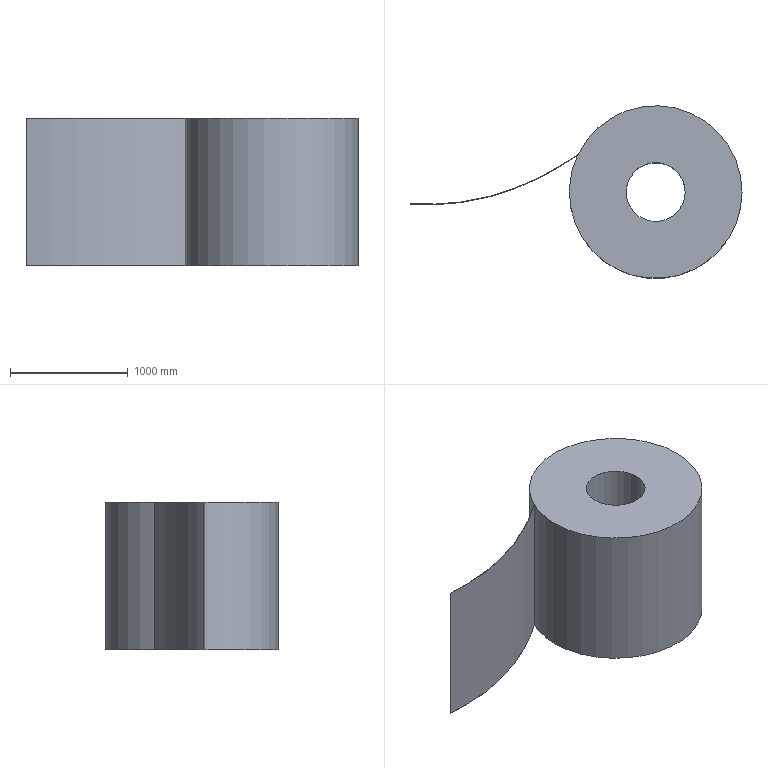Part | SolidWorks | features ExtruThin 1, ICE 1 | 1 solid | 10 faces | box 2820 x 1466 x 1250 mm | volume 1870768700 mm3 | cylinder 5 | plane 3 | spline 2 | commonest cylinder face diameters 1466 x3 500 x2
STEP:
#1=CARTESIAN_POINT('',(3099.7,210.,-625.));
#2=VERTEX_POINT('',#1);
#3=CARTESIAN_POINT('',(2599.7,210.,-625.));
#4=VERTEX_POINT('',#3);
#5=CARTESIAN_POINT('',(2849.7,210.,-625.));
#6=DIRECTION('',(0.,0.,-1.));
#7=DIRECTION('',(1.,0.,0.));
#8=AXIS2_PLACEMENT_3D('',#5,#6,#7);
#9=CIRCLE('',#8,250.);
#10=EDGE_CURVE('',#2,#4,#9,.T.);
#11=ORIENTED_EDGE('',*,*,#10,.T.);
#12=CARTESIAN_POINT('',(2599.7,210.,625.));
#13=VERTEX_POINT('',#12);
#14=CARTESIAN_POINT('',(2599.7,210.,-2698.525));
#15=DIRECTION('',(0.,0.,1.));
#16=VECTOR('',#15,1000.);
#17=LINE('',#14,#16);
#18=EDGE_CURVE('',#4,#13,#17,.T.);
#19=ORIENTED_EDGE('',*,*,#18,.T.);
#20=CARTESIAN_POINT('',(3099.7,210.,625.));
#21=VERTEX_POINT('',#20);
#22=CARTESIAN_POINT('',(2849.7,210.,625.));
#23=DIRECTION('',(0.,0.,1.));
#24=DIRECTION('',(1.,0.,0.));
#25=AXIS2_PLACEMENT_3D('',#22,#23,#24);
#26=CIRCLE('',#25,250.);
#27=EDGE_CURVE('',#13,#21,#26,.T.);
#28=ORIENTED_EDGE('',*,*,#27,.T.);
#29=CARTESIAN_POINT('',(3099.7,210.,-2698.525));
#30=DIRECTION('',(0.,0.,1.));
#31=VECTOR('',#30,1000.);
#32=LINE('',#29,#31);
#33=EDGE_CURVE('',#2,#21,#32,.T.);
#34=ORIENTED_EDGE('',*,*,#33,.F.);
#35=EDGE_LOOP('',(#11,#19,#28,#34));
#36=FACE_OUTER_BOUND('',#35,.T.);
#37=CARTESIAN_POINT('',(2849.7,210.,-2698.525));
#38=DIRECTION('',(0.,0.,1.));
#39=DIRECTION('',(1.,0.,0.));
#40=AXIS2_PLACEMENT_3D('',#37,#38,#39);
#41=CYLINDRICAL_SURFACE('',#40,250.);
#42=ADVANCED_FACE('',(#36),#41,.F.);
#43=CARTESIAN_POINT('',(2116.598,210.,-625.));
#44=VERTEX_POINT('',#43);
#45=CARTESIAN_POINT('',(2188.389,526.395,-625.));
#46=VERTEX_POINT('',#45);
#47=CARTESIAN_POINT('',(2849.7,210.,-625.));
#48=DIRECTION('',(0.,0.,-1.));
#49=DIRECTION('',(1.,0.,0.));
#50=AXIS2_PLACEMENT_3D('',#47,#48,#49);
#51=CIRCLE('',#50,733.102);
#52=EDGE_CURVE('',#44,#46,#51,.T.);
#53=ORIENTED_EDGE('',*,*,#52,.F.);
#54=CARTESIAN_POINT('',(2116.598,210.,625.));
#55=VERTEX_POINT('',#54);
#56=CARTESIAN_POINT('',(2116.598,210.,-2698.525));
#57=DIRECTION('',(0.,0.,1.));
#58=VECTOR('',#57,1000.);
#59=LINE('',#56,#58);
#60=EDGE_CURVE('',#44,#55,#59,.T.);
#61=ORIENTED_EDGE('',*,*,#60,.T.);
#62=CARTESIAN_POINT('',(2188.389,526.395,625.));
#63=VERTEX_POINT('',#62);
#64=CARTESIAN_POINT('',(2849.7,210.,625.));
#65=DIRECTION('',(0.,0.,1.));
#66=DIRECTION('',(1.,0.,0.));
#67=AXIS2_PLACEMENT_3D('',#64,#65,#66);
#68=CIRCLE('',#67,733.102);
#69=EDGE_CURVE('',#63,#55,#68,.T.);
#70=ORIENTED_EDGE('',*,*,#69,.F.);
#71=CARTESIAN_POINT('',(2188.389,526.395,625.));
#72=DIRECTION('',(0.,0.,1.));
#73=VECTOR('',#72,1000.);
#74=LINE('',#71,#73);
#75=EDGE_CURVE('',#46,#63,#74,.T.);
#76=ORIENTED_EDGE('',*,*,#75,.F.);
#77=EDGE_LOOP('',(#53,#61,#70,#76));
#78=FACE_OUTER_BOUND('',#77,.T.);
#79=CARTESIAN_POINT('',(2849.7,210.,-2698.525));
#80=DIRECTION('',(0.,0.,1.));
#81=DIRECTION('',(1.,0.,0.));
#82=AXIS2_PLACEMENT_3D('',#79,#80,#81);
#83=CYLINDRICAL_SURFACE('',#82,733.102);
#84=ADVANCED_FACE('',(#78),#83,.T.);
#85=ORIENTED_EDGE('',*,*,#60,.F.);
#86=CARTESIAN_POINT('',(3582.802,210.,-625.));
#87=VERTEX_POINT('',#86);
#88=CARTESIAN_POINT('',(2849.7,210.,-625.));
#89=DIRECTION('',(0.,0.,-1.));
#90=DIRECTION('',(1.,0.,0.));
#91=AXIS2_PLACEMENT_3D('',#88,#89,#90);
#92=CIRCLE('',#91,733.102);
#93=EDGE_CURVE('',#87,#44,#92,.T.);
#94=ORIENTED_EDGE('',*,*,#93,.F.);
#95=CARTESIAN_POINT('',(3582.802,210.,625.));
#96=VERTEX_POINT('',#95);
#97=CARTESIAN_POINT('',(3582.802,210.,-2698.525));
#98=DIRECTION('',(0.,0.,1.));
#99=VECTOR('',#98,1000.);
#100=LINE('',#97,#99);
#101=EDGE_CURVE('',#87,#96,#100,.T.);
#102=ORIENTED_EDGE('',*,*,#101,.T.);
#103=CARTESIAN_POINT('',(2849.7,210.,625.));
#104=DIRECTION('',(0.,0.,1.));
#105=DIRECTION('',(1.,0.,0.));
#106=AXIS2_PLACEMENT_3D('',#103,#104,#105);
#107=CIRCLE('',#106,733.102);
#108=EDGE_CURVE('',#55,#96,#107,.T.);
#109=ORIENTED_EDGE('',*,*,#108,.F.);
#110=EDGE_LOOP('',(#85,#94,#102,#109));
#111=FACE_OUTER_BOUND('',#110,.T.);
#112=CARTESIAN_POINT('',(2849.7,210.,-2698.525));
#113=DIRECTION('',(0.,0.,1.));
#114=DIRECTION('',(1.,0.,0.));
#115=AXIS2_PLACEMENT_3D('',#112,#113,#114);
#116=CYLINDRICAL_SURFACE('',#115,733.102);
#117=ADVANCED_FACE('',(#111),#116,.T.);
#118=CARTESIAN_POINT('',(762.74,109.82,-625.));
#119=VERTEX_POINT('',#118);
#120=CARTESIAN_POINT('',(762.74,109.82,-625.));
#121=CARTESIAN_POINT('',(1013.548,91.191,-625.));
#122=CARTESIAN_POINT('',(1258.171,116.87,-625.));
#123=CARTESIAN_POINT('',(1733.318,256.354,-625.));
#124=CARTESIAN_POINT('',(1963.927,369.542,-625.));
#125=CARTESIAN_POINT('',(2188.389,526.395,-625.));
#126=B_SPLINE_CURVE_WITH_KNOTS('',3,(#120,#121,#122,#123,#124,#125),.UNSPECIFIED.,.F.,.F.,(4,2,4),(0.,0.5,0.9965),.UNSPECIFIED.);
#127=EDGE_CURVE('',#119,#46,#126,.T.);
#128=ORIENTED_EDGE('',*,*,#127,.T.);
#129=ORIENTED_EDGE('',*,*,#75,.T.);
#130=CARTESIAN_POINT('',(762.74,109.82,625.));
#131=VERTEX_POINT('',#130);
#132=CARTESIAN_POINT('',(762.74,109.82,625.));
#133=CARTESIAN_POINT('',(1013.548,91.191,625.));
#134=CARTESIAN_POINT('',(1258.171,116.87,625.));
#135=CARTESIAN_POINT('',(1733.318,256.354,625.));
#136=CARTESIAN_POINT('',(1963.927,369.542,625.));
#137=CARTESIAN_POINT('',(2188.389,526.395,625.));
#138=B_SPLINE_CURVE_WITH_KNOTS('',3,(#132,#133,#134,#135,#136,#137),.UNSPECIFIED.,.F.,.F.,(4,2,4),(0.,0.5,0.9965),.UNSPECIFIED.);
#139=EDGE_CURVE('',#131,#63,#138,.T.);
#140=ORIENTED_EDGE('',*,*,#139,.F.);
#141=CARTESIAN_POINT('',(762.74,109.82,625.));
#142=DIRECTION('',(0.,0.,-1.));
#143=VECTOR('',#142,1000.);
#144=LINE('',#141,#143);
#145=EDGE_CURVE('',#131,#119,#144,.T.);
#146=ORIENTED_EDGE('',*,*,#145,.T.);
#147=EDGE_LOOP('',(#128,#129,#140,#146));
#148=FACE_OUTER_BOUND('',#147,.T.);
#149=CARTESIAN_POINT('',(762.74,109.82,625.));
#150=CARTESIAN_POINT('',(762.74,109.82,-625.));
#151=CARTESIAN_POINT('',(1013.548,91.191,625.));
#152=CARTESIAN_POINT('',(1013.548,91.191,-625.));
#153=CARTESIAN_POINT('',(1258.171,116.87,625.));
#154=CARTESIAN_POINT('',(1258.171,116.87,-625.));
#155=CARTESIAN_POINT('',(1733.318,256.354,625.));
#156=CARTESIAN_POINT('',(1733.318,256.354,-625.));
#157=CARTESIAN_POINT('',(1963.927,369.542,625.));
#158=CARTESIAN_POINT('',(1963.927,369.542,-625.));
#159=CARTESIAN_POINT('',(2188.389,526.395,625.));
#160=CARTESIAN_POINT('',(2188.389,526.395,-625.));
#161=B_SPLINE_SURFACE_WITH_KNOTS('',3,1,((#149,#150),(#151,#152),(#153,#154),(#155,#156),(#157,#158),(#159,#160)),.UNSPECIFIED.,.F.,.F.,.F.,(4,2,4),(2,2),(0.,0.5,0.9965),(0.,1.),.UNSPECIFIED.);
#162=ADVANCED_FACE('',(#148),#161,.F.);
#163=CARTESIAN_POINT('',(2191.067,531.933,-625.));
#164=VERTEX_POINT('',#163);
#165=CARTESIAN_POINT('',(2191.067,531.933,625.));
#166=VERTEX_POINT('',#165);
#167=CARTESIAN_POINT('',(2191.067,531.933,625.));
#168=DIRECTION('',(0.,0.,1.));
#169=VECTOR('',#168,1000.);
#170=LINE('',#167,#169);
#171=EDGE_CURVE('',#164,#166,#170,.T.);
#172=ORIENTED_EDGE('',*,*,#171,.F.);
#173=CARTESIAN_POINT('',(762.962,112.812,-625.));
#174=VERTEX_POINT('',#173);
#175=CARTESIAN_POINT('',(762.962,112.812,-625.));
#176=CARTESIAN_POINT('',(1013.423,94.209,-625.));
#177=CARTESIAN_POINT('',(1257.667,119.849,-625.));
#178=CARTESIAN_POINT('',(1733.679,259.586,-625.));
#179=CARTESIAN_POINT('',(1965.455,373.645,-625.));
#180=CARTESIAN_POINT('',(2191.067,531.933,-625.));
#181=B_SPLINE_CURVE_WITH_KNOTS('',3,(#175,#176,#177,#178,#179,#180),.UNSPECIFIED.,.F.,.F.,(4,2,4),(0.,0.5,0.9998),.UNSPECIFIED.);
#182=EDGE_CURVE('',#174,#164,#181,.T.);
#183=ORIENTED_EDGE('',*,*,#182,.F.);
#184=CARTESIAN_POINT('',(762.962,112.812,625.));
#185=VERTEX_POINT('',#184);
#186=CARTESIAN_POINT('',(762.962,112.812,625.));
#187=DIRECTION('',(0.,0.,-1.));
#188=VECTOR('',#187,1000.);
#189=LINE('',#186,#188);
#190=EDGE_CURVE('',#185,#174,#189,.T.);
#191=ORIENTED_EDGE('',*,*,#190,.F.);
#192=CARTESIAN_POINT('',(762.962,112.812,625.));
#193=CARTESIAN_POINT('',(1013.423,94.209,625.));
#194=CARTESIAN_POINT('',(1257.667,119.849,625.));
#195=CARTESIAN_POINT('',(1733.679,259.586,625.));
#196=CARTESIAN_POINT('',(1965.455,373.645,625.));
#197=CARTESIAN_POINT('',(2191.067,531.933,625.));
#198=B_SPLINE_CURVE_WITH_KNOTS('',3,(#192,#193,#194,#195,#196,#197),.UNSPECIFIED.,.F.,.F.,(4,2,4),(0.,0.5,0.9998),.UNSPECIFIED.);
#199=EDGE_CURVE('',#185,#166,#198,.T.);
#200=ORIENTED_EDGE('',*,*,#199,.T.);
#201=EDGE_LOOP('',(#172,#183,#191,#200));
#202=FACE_OUTER_BOUND('',#201,.T.);
#203=CARTESIAN_POINT('',(762.962,112.812,625.));
#204=CARTESIAN_POINT('',(762.962,112.812,-625.));
#205=CARTESIAN_POINT('',(1013.423,94.209,625.));
#206=CARTESIAN_POINT('',(1013.423,94.209,-625.));
#207=CARTESIAN_POINT('',(1257.667,119.849,625.));
#208=CARTESIAN_POINT('',(1257.667,119.849,-625.));
#209=CARTESIAN_POINT('',(1733.679,259.586,625.));
#210=CARTESIAN_POINT('',(1733.679,259.586,-625.));
#211=CARTESIAN_POINT('',(1965.455,373.645,625.));
#212=CARTESIAN_POINT('',(1965.455,373.645,-625.));
#213=CARTESIAN_POINT('',(2191.067,531.933,625.));
#214=CARTESIAN_POINT('',(2191.067,531.933,-625.));
#215=B_SPLINE_SURFACE_WITH_KNOTS('',3,1,((#203,#204),(#205,#206),(#207,#208),(#209,#210),(#211,#212),(#213,#214)),.UNSPECIFIED.,.F.,.F.,.F.,(4,2,4),(2,2),(0.,0.5,0.9998),(0.,1.),.UNSPECIFIED.);
#216=ADVANCED_FACE('',(#202),#215,.T.);
#217=CARTESIAN_POINT('',(762.74,109.82,-625.));
#218=DIRECTION('',(0.07407,0.9973,0.));
#219=VECTOR('',#218,1000.);
#220=LINE('',#217,#219);
#221=EDGE_CURVE('',#119,#174,#220,.T.);
#222=ORIENTED_EDGE('',*,*,#221,.F.);
#223=ORIENTED_EDGE('',*,*,#145,.F.);
#224=CARTESIAN_POINT('',(762.74,109.82,625.));
#225=DIRECTION('',(0.07407,0.9973,0.));
#226=VECTOR('',#225,1000.);
#227=LINE('',#224,#226);
#228=EDGE_CURVE('',#131,#185,#227,.T.);
#229=ORIENTED_EDGE('',*,*,#228,.T.);
#230=ORIENTED_EDGE('',*,*,#190,.T.);
#231=EDGE_LOOP('',(#222,#223,#229,#230));
#232=FACE_OUTER_BOUND('',#231,.T.);
#233=CARTESIAN_POINT('',(762.74,109.82,625.));
#234=DIRECTION('',(-0.9973,0.07407,0.));
#235=DIRECTION('',(-0.07407,-0.9973,0.));
#236=AXIS2_PLACEMENT_3D('',#233,#234,#235);
#237=PLANE('',#236);
#238=ADVANCED_FACE('',(#232),#237,.T.);
#239=ORIENTED_EDGE('',*,*,#139,.T.);
#240=ORIENTED_EDGE('',*,*,#69,.T.);
#241=ORIENTED_EDGE('',*,*,#108,.T.);
#242=CARTESIAN_POINT('',(2849.7,210.,625.));
#243=DIRECTION('',(0.,0.,1.));
#244=DIRECTION('',(1.,0.,0.));
#245=AXIS2_PLACEMENT_3D('',#242,#243,#244);
#246=CIRCLE('',#245,733.102);
#247=EDGE_CURVE('',#96,#166,#246,.T.);
#248=ORIENTED_EDGE('',*,*,#247,.T.);
#249=ORIENTED_EDGE('',*,*,#199,.F.);
#250=ORIENTED_EDGE('',*,*,#228,.F.);
#251=EDGE_LOOP('',(#239,#240,#241,#248,#249,#250));
#252=FACE_OUTER_BOUND('',#251,.T.);
#253=CARTESIAN_POINT('',(2849.7,210.,625.));
#254=DIRECTION('',(0.,0.,1.));
#255=DIRECTION('',(1.,0.,0.));
#256=AXIS2_PLACEMENT_3D('',#253,#254,#255);
#257=CIRCLE('',#256,250.);
#258=EDGE_CURVE('',#21,#13,#257,.T.);
#259=ORIENTED_EDGE('',*,*,#258,.F.);
#260=ORIENTED_EDGE('',*,*,#27,.F.);
#261=EDGE_LOOP('',(#259,#260));
#262=FACE_BOUND('',#261,.T.);
#263=CARTESIAN_POINT('',(1496.574,186.856,625.));
#264=DIRECTION('',(0.,0.,-1.));
#265=DIRECTION('',(-1.,0.,0.));
#266=AXIS2_PLACEMENT_3D('',#263,#264,#265);
#267=PLANE('',#266);
#268=ADVANCED_FACE('',(#252,#262),#267,.F.);
#269=ORIENTED_EDGE('',*,*,#182,.T.);
#270=CARTESIAN_POINT('',(2849.7,210.,-625.));
#271=DIRECTION('',(0.,0.,-1.));
#272=DIRECTION('',(1.,0.,0.));
#273=AXIS2_PLACEMENT_3D('',#270,#271,#272);
#274=CIRCLE('',#273,733.102);
#275=EDGE_CURVE('',#164,#87,#274,.T.);
#276=ORIENTED_EDGE('',*,*,#275,.T.);
#277=ORIENTED_EDGE('',*,*,#93,.T.);
#278=ORIENTED_EDGE('',*,*,#52,.T.);
#279=ORIENTED_EDGE('',*,*,#127,.F.);
#280=ORIENTED_EDGE('',*,*,#221,.T.);
#281=EDGE_LOOP('',(#269,#276,#277,#278,#279,#280));
#282=FACE_OUTER_BOUND('',#281,.T.);
#283=ORIENTED_EDGE('',*,*,#10,.F.);
#284=CARTESIAN_POINT('',(2849.7,210.,-625.));
#285=DIRECTION('',(0.,0.,-1.));
#286=DIRECTION('',(1.,0.,0.));
#287=AXIS2_PLACEMENT_3D('',#284,#285,#286);
#288=CIRCLE('',#287,250.);
#289=EDGE_CURVE('',#4,#2,#288,.T.);
#290=ORIENTED_EDGE('',*,*,#289,.F.);
#291=EDGE_LOOP('',(#283,#290));
#292=FACE_BOUND('',#291,.T.);
#293=CARTESIAN_POINT('',(1496.574,186.856,-625.));
#294=DIRECTION('',(0.,0.,-1.));
#295=DIRECTION('',(-1.,0.,0.));
#296=AXIS2_PLACEMENT_3D('',#293,#294,#295);
#297=PLANE('',#296);
#298=ADVANCED_FACE('',(#282,#292),#297,.T.);
#299=ORIENTED_EDGE('',*,*,#101,.F.);
#300=ORIENTED_EDGE('',*,*,#275,.F.);
#301=ORIENTED_EDGE('',*,*,#171,.T.);
#302=ORIENTED_EDGE('',*,*,#247,.F.);
#303=EDGE_LOOP('',(#299,#300,#301,#302));
#304=FACE_OUTER_BOUND('',#303,.T.);
#305=CARTESIAN_POINT('',(2849.7,210.,-2698.525));
#306=DIRECTION('',(0.,0.,1.));
#307=DIRECTION('',(1.,0.,0.));
#308=AXIS2_PLACEMENT_3D('',#305,#306,#307);
#309=CYLINDRICAL_SURFACE('',#308,733.102);
#310=ADVANCED_FACE('',(#304),#309,.T.);
#311=ORIENTED_EDGE('',*,*,#18,.F.);
#312=ORIENTED_EDGE('',*,*,#289,.T.);
#313=ORIENTED_EDGE('',*,*,#33,.T.);
#314=ORIENTED_EDGE('',*,*,#258,.T.);
#315=EDGE_LOOP('',(#311,#312,#313,#314));
#316=FACE_OUTER_BOUND('',#315,.T.);
#317=CARTESIAN_POINT('',(2849.7,210.,-2698.525));
#318=DIRECTION('',(0.,0.,1.));
#319=DIRECTION('',(1.,0.,0.));
#320=AXIS2_PLACEMENT_3D('',#317,#318,#319);
#321=CYLINDRICAL_SURFACE('',#320,250.);
#322=ADVANCED_FACE('',(#316),#321,.F.);
#323=CLOSED_SHELL('',(#42,#84,#117,#162,#216,#238,#268,#298,#310,#322));
#324=MANIFOLD_SOLID_BREP('',#323);
#325=CARTESIAN_POINT('',(0.,0.,0.));
#326=DIRECTION('',(0.,0.,1.));
#327=DIRECTION('',(1.,0.,0.));
#328=AXIS2_PLACEMENT_3D('',#325,#326,#327);
#329=(LENGTH_UNIT()NAMED_UNIT(*)SI_UNIT(.MILLI.,.METRE.));
#330=UNCERTAINTY_MEASURE_WITH_UNIT(LENGTH_MEASURE(0.00001),#329,'','');
#331=(NAMED_UNIT(*)PLANE_ANGLE_UNIT()SI_UNIT($,.RADIAN.));
#332=(NAMED_UNIT(*)SI_UNIT($,.STERADIAN.)SOLID_ANGLE_UNIT());
#333=(GEOMETRIC_REPRESENTATION_CONTEXT(3)GLOBAL_UNCERTAINTY_ASSIGNED_CONTEXT((#330))GLOBAL_UNIT_ASSIGNED_CONTEXT((#329,#331,#332))REPRESENTATION_CONTEXT('',''));
#334=ADVANCED_BREP_SHAPE_REPRESENTATION('',(#324,#328),#333);